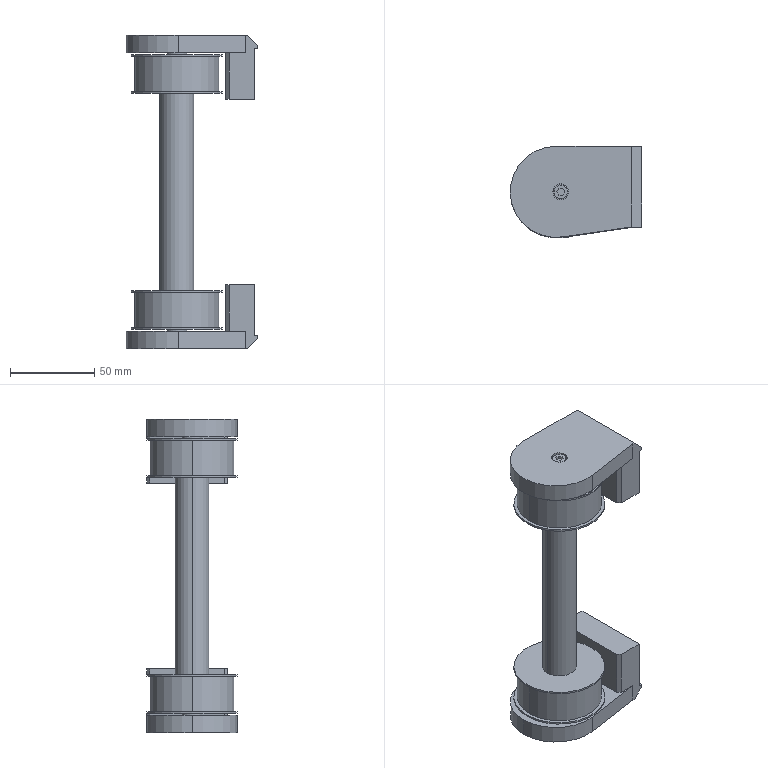Part | STEP file | Guide wheel mechanism revised.sldasm-Part-82 | 1 solid | 189 faces | box 78 x 54 x 186 mm | volume 247289 mm3 | plane 148 | cylinder 37 | cone 4 | commonest cylinder face diameters 54 x11 5 x8 8.5 x4 9.5 x4 12 x4 50 x4